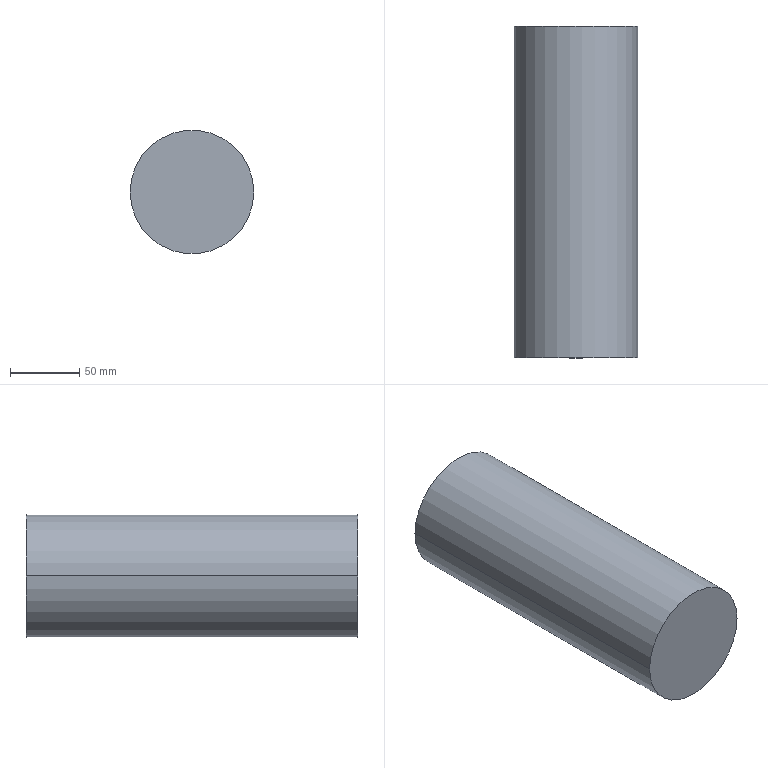Part | STEP file | 1 solid | 7 faces | box 89.417 x 240 x 89.417 mm | volume 636634 mm3 | cylinder 4 | plane 3 | commonest cylinder face diameters 69.417 x2 89.417 x2
STEP:
#1=CARTESIAN_POINT('',(0.,0.,0.));
#2=DIRECTION('',(0.,0.,1.));
#3=DIRECTION('',(1.,0.,0.));
#4=AXIS2_PLACEMENT_3D('',#1,#2,#3);
#5=CARTESIAN_POINT('',(677.16,51.164,248.078));
#6=VERTEX_POINT('',#5);
#7=CARTESIAN_POINT('',(677.16,-178.836,248.078));
#8=VERTEX_POINT('',#7);
#9=CARTESIAN_POINT('',(677.16,51.164,248.078));
#10=DIRECTION('',(0.,-1.,0.));
#11=VECTOR('',#10,1.);
#12=LINE('',#9,#11);
#13=CARTESIAN_POINT('',(642.452,51.164,248.078));
#14=DIRECTION('',(0.,-1.,0.));
#15=DIRECTION('',(1.,0.,0.));
#16=AXIS2_PLACEMENT_3D('',#13,#14,#15);
#17=CYLINDRICAL_SURFACE('',#16,34.708);
#18=CARTESIAN_POINT('',(6.283,0.));
#19=DIRECTION('',(0.,1.));
#20=VECTOR('',#19,1.);
#21=LINE('',#18,#20);
#22=(GEOMETRIC_REPRESENTATION_CONTEXT(2)PARAMETRIC_REPRESENTATION_CONTEXT()REPRESENTATION_CONTEXT('',''));
#23=DEFINITIONAL_REPRESENTATION('',(#21),#22);
#24=PCURVE('',#17,#23);
#25=CARTESIAN_POINT('',(642.452,51.164,248.078));
#26=DIRECTION('',(0.,-1.,0.));
#27=DIRECTION('',(1.,0.,0.));
#28=AXIS2_PLACEMENT_3D('',#25,#26,#27);
#29=CYLINDRICAL_SURFACE('',#28,34.708);
#30=CARTESIAN_POINT('',(0.,0.));
#31=DIRECTION('',(0.,1.));
#32=VECTOR('',#31,1.);
#33=LINE('',#30,#32);
#34=(GEOMETRIC_REPRESENTATION_CONTEXT(2)PARAMETRIC_REPRESENTATION_CONTEXT()REPRESENTATION_CONTEXT('',''));
#35=DEFINITIONAL_REPRESENTATION('',(#33),#34);
#36=PCURVE('',#29,#35);
#37=SURFACE_CURVE('',#12,(#24,#36),.PCURVE_S1.);
#38=EDGE_CURVE('',#6,#8,#37,.T.);
#39=ORIENTED_EDGE('',*,*,#38,.T.);
#40=CARTESIAN_POINT('',(607.743,-178.836,248.078));
#41=VERTEX_POINT('',#40);
#42=CARTESIAN_POINT('',(642.452,-178.836,248.078));
#43=DIRECTION('',(0.,1.,0.));
#44=DIRECTION('',(-1.,0.,0.));
#45=AXIS2_PLACEMENT_3D('',#42,#43,#44);
#46=CIRCLE('',#45,34.708);
#47=CARTESIAN_POINT('',(9.425,230.));
#48=DIRECTION('',(-1.,0.));
#49=VECTOR('',#48,1.);
#50=LINE('',#47,#49);
#51=(GEOMETRIC_REPRESENTATION_CONTEXT(2)PARAMETRIC_REPRESENTATION_CONTEXT()REPRESENTATION_CONTEXT('',''));
#52=DEFINITIONAL_REPRESENTATION('',(#50),#51);
#53=PCURVE('',#17,#52);
#54=CARTESIAN_POINT('',(642.452,-178.836,248.078));
#55=DIRECTION('',(0.,1.,0.));
#56=DIRECTION('',(-1.,0.,0.));
#57=AXIS2_PLACEMENT_3D('',#54,#55,#56);
#58=PLANE('',#57);
#59=CARTESIAN_POINT('',(0.,0.));
#60=DIRECTION('',(1.,0.));
#61=AXIS2_PLACEMENT_2D('',#59,#60);
#62=CIRCLE('',#61,34.708);
#63=(GEOMETRIC_REPRESENTATION_CONTEXT(2)PARAMETRIC_REPRESENTATION_CONTEXT()REPRESENTATION_CONTEXT('',''));
#64=DEFINITIONAL_REPRESENTATION('',(#62),#63);
#65=PCURVE('',#58,#64);
#66=SURFACE_CURVE('',#46,(#53,#65),.PCURVE_S1.);
#67=EDGE_CURVE('',#8,#41,#66,.T.);
#68=ORIENTED_EDGE('',*,*,#67,.T.);
#69=CARTESIAN_POINT('',(607.743,51.164,248.078));
#70=VERTEX_POINT('',#69);
#71=CARTESIAN_POINT('',(607.743,51.164,248.078));
#72=DIRECTION('',(0.,-1.,0.));
#73=VECTOR('',#72,1.);
#74=LINE('',#71,#73);
#75=CARTESIAN_POINT('',(3.142,0.));
#76=DIRECTION('',(0.,1.));
#77=VECTOR('',#76,1.);
#78=LINE('',#75,#77);
#79=(GEOMETRIC_REPRESENTATION_CONTEXT(2)PARAMETRIC_REPRESENTATION_CONTEXT()REPRESENTATION_CONTEXT('',''));
#80=DEFINITIONAL_REPRESENTATION('',(#78),#79);
#81=PCURVE('',#17,#80);
#82=CARTESIAN_POINT('',(3.142,0.));
#83=DIRECTION('',(0.,1.));
#84=VECTOR('',#83,1.);
#85=LINE('',#82,#84);
#86=(GEOMETRIC_REPRESENTATION_CONTEXT(2)PARAMETRIC_REPRESENTATION_CONTEXT()REPRESENTATION_CONTEXT('',''));
#87=DEFINITIONAL_REPRESENTATION('',(#85),#86);
#88=PCURVE('',#29,#87);
#89=SURFACE_CURVE('',#74,(#81,#88),.PCURVE_S1.);
#90=EDGE_CURVE('',#70,#41,#89,.T.);
#91=ORIENTED_EDGE('',*,*,#90,.F.);
#92=CARTESIAN_POINT('',(642.452,51.164,248.078));
#93=DIRECTION('',(0.,1.,0.));
#94=DIRECTION('',(-1.,0.,0.));
#95=AXIS2_PLACEMENT_3D('',#92,#93,#94);
#96=CIRCLE('',#95,34.708);
#97=CARTESIAN_POINT('',(9.425,0.));
#98=DIRECTION('',(-1.,0.));
#99=VECTOR('',#98,1.);
#100=LINE('',#97,#99);
#101=(GEOMETRIC_REPRESENTATION_CONTEXT(2)PARAMETRIC_REPRESENTATION_CONTEXT()REPRESENTATION_CONTEXT('',''));
#102=DEFINITIONAL_REPRESENTATION('',(#100),#101);
#103=PCURVE('',#17,#102);
#104=CARTESIAN_POINT('',(642.452,51.164,248.078));
#105=DIRECTION('',(0.,1.,0.));
#106=DIRECTION('',(-1.,0.,0.));
#107=AXIS2_PLACEMENT_3D('',#104,#105,#106);
#108=PLANE('',#107);
#109=CARTESIAN_POINT('',(0.,0.));
#110=DIRECTION('',(1.,0.));
#111=AXIS2_PLACEMENT_2D('',#109,#110);
#112=CIRCLE('',#111,34.708);
#113=(GEOMETRIC_REPRESENTATION_CONTEXT(2)PARAMETRIC_REPRESENTATION_CONTEXT()REPRESENTATION_CONTEXT('',''));
#114=DEFINITIONAL_REPRESENTATION('',(#112),#113);
#115=PCURVE('',#108,#114);
#116=SURFACE_CURVE('',#96,(#103,#115),.PCURVE_S1.);
#117=EDGE_CURVE('',#6,#70,#116,.T.);
#118=ORIENTED_EDGE('',*,*,#117,.F.);
#119=EDGE_LOOP('',(#39,#68,#91,#118));
#120=FACE_BOUND('',#119,.F.);
#121=ADVANCED_FACE('',(#120),#17,.F.);
#122=CARTESIAN_POINT('',(597.743,51.164,248.078));
#123=VERTEX_POINT('',#122);
#124=CARTESIAN_POINT('',(687.16,51.164,248.078));
#125=VERTEX_POINT('',#124);
#126=CARTESIAN_POINT('',(642.452,51.164,248.078));
#127=DIRECTION('',(0.,1.,0.));
#128=DIRECTION('',(-1.,0.,0.));
#129=AXIS2_PLACEMENT_3D('',#126,#127,#128);
#130=CIRCLE('',#129,44.708);
#131=CARTESIAN_POINT('',(642.452,51.164,248.078));
#132=DIRECTION('',(0.,-1.,0.));
#133=DIRECTION('',(1.,0.,0.));
#134=AXIS2_PLACEMENT_3D('',#131,#132,#133);
#135=CYLINDRICAL_SURFACE('',#134,44.708);
#136=CARTESIAN_POINT('',(3.142,0.));
#137=DIRECTION('',(-1.,0.));
#138=VECTOR('',#137,1.);
#139=LINE('',#136,#138);
#140=(GEOMETRIC_REPRESENTATION_CONTEXT(2)PARAMETRIC_REPRESENTATION_CONTEXT()REPRESENTATION_CONTEXT('',''));
#141=DEFINITIONAL_REPRESENTATION('',(#139),#140);
#142=PCURVE('',#135,#141);
#143=CARTESIAN_POINT('',(0.,0.));
#144=DIRECTION('',(1.,0.));
#145=AXIS2_PLACEMENT_2D('',#143,#144);
#146=CIRCLE('',#145,44.708);
#147=(GEOMETRIC_REPRESENTATION_CONTEXT(2)PARAMETRIC_REPRESENTATION_CONTEXT()REPRESENTATION_CONTEXT('',''));
#148=DEFINITIONAL_REPRESENTATION('',(#146),#147);
#149=PCURVE('',#108,#148);
#150=SURFACE_CURVE('',#130,(#142,#149),.PCURVE_S1.);
#151=EDGE_CURVE('',#123,#125,#150,.T.);
#152=ORIENTED_EDGE('',*,*,#151,.F.);
#153=CARTESIAN_POINT('',(597.743,-188.836,248.078));
#154=VERTEX_POINT('',#153);
#155=CARTESIAN_POINT('',(597.743,51.164,248.078));
#156=DIRECTION('',(0.,-1.,0.));
#157=VECTOR('',#156,1.);
#158=LINE('',#155,#157);
#159=CARTESIAN_POINT('',(3.142,0.));
#160=DIRECTION('',(0.,1.));
#161=VECTOR('',#160,1.);
#162=LINE('',#159,#161);
#163=(GEOMETRIC_REPRESENTATION_CONTEXT(2)PARAMETRIC_REPRESENTATION_CONTEXT()REPRESENTATION_CONTEXT('',''));
#164=DEFINITIONAL_REPRESENTATION('',(#162),#163);
#165=PCURVE('',#135,#164);
#166=CARTESIAN_POINT('',(642.452,51.164,248.078));
#167=DIRECTION('',(0.,-1.,0.));
#168=DIRECTION('',(1.,0.,0.));
#169=AXIS2_PLACEMENT_3D('',#166,#167,#168);
#170=CYLINDRICAL_SURFACE('',#169,44.708);
#171=CARTESIAN_POINT('',(3.142,0.));
#172=DIRECTION('',(0.,1.));
#173=VECTOR('',#172,1.);
#174=LINE('',#171,#173);
#175=(GEOMETRIC_REPRESENTATION_CONTEXT(2)PARAMETRIC_REPRESENTATION_CONTEXT()REPRESENTATION_CONTEXT('',''));
#176=DEFINITIONAL_REPRESENTATION('',(#174),#175);
#177=PCURVE('',#170,#176);
#178=SURFACE_CURVE('',#158,(#165,#177),.PCURVE_S1.);
#179=EDGE_CURVE('',#123,#154,#178,.T.);
#180=ORIENTED_EDGE('',*,*,#179,.T.);
#181=CARTESIAN_POINT('',(687.16,-188.836,248.078));
#182=VERTEX_POINT('',#181);
#183=CARTESIAN_POINT('',(642.452,-188.836,248.078));
#184=DIRECTION('',(0.,1.,0.));
#185=DIRECTION('',(-1.,0.,0.));
#186=AXIS2_PLACEMENT_3D('',#183,#184,#185);
#187=CIRCLE('',#186,44.708);
#188=CARTESIAN_POINT('',(3.142,240.));
#189=DIRECTION('',(-1.,0.));
#190=VECTOR('',#189,1.);
#191=LINE('',#188,#190);
#192=(GEOMETRIC_REPRESENTATION_CONTEXT(2)PARAMETRIC_REPRESENTATION_CONTEXT()REPRESENTATION_CONTEXT('',''));
#193=DEFINITIONAL_REPRESENTATION('',(#191),#192);
#194=PCURVE('',#135,#193);
#195=CARTESIAN_POINT('',(642.452,-188.836,248.078));
#196=DIRECTION('',(0.,1.,0.));
#197=DIRECTION('',(-1.,0.,0.));
#198=AXIS2_PLACEMENT_3D('',#195,#196,#197);
#199=PLANE('',#198);
#200=CARTESIAN_POINT('',(0.,0.));
#201=DIRECTION('',(1.,0.));
#202=AXIS2_PLACEMENT_2D('',#200,#201);
#203=CIRCLE('',#202,44.708);
#204=(GEOMETRIC_REPRESENTATION_CONTEXT(2)PARAMETRIC_REPRESENTATION_CONTEXT()REPRESENTATION_CONTEXT('',''));
#205=DEFINITIONAL_REPRESENTATION('',(#203),#204);
#206=PCURVE('',#199,#205);
#207=SURFACE_CURVE('',#187,(#194,#206),.PCURVE_S1.);
#208=EDGE_CURVE('',#154,#182,#207,.T.);
#209=ORIENTED_EDGE('',*,*,#208,.T.);
#210=CARTESIAN_POINT('',(687.16,51.164,248.078));
#211=DIRECTION('',(0.,-1.,0.));
#212=VECTOR('',#211,1.);
#213=LINE('',#210,#212);
#214=CARTESIAN_POINT('',(0.,0.));
#215=DIRECTION('',(0.,1.));
#216=VECTOR('',#215,1.);
#217=LINE('',#214,#216);
#218=(GEOMETRIC_REPRESENTATION_CONTEXT(2)PARAMETRIC_REPRESENTATION_CONTEXT()REPRESENTATION_CONTEXT('',''));
#219=DEFINITIONAL_REPRESENTATION('',(#217),#218);
#220=PCURVE('',#135,#219);
#221=CARTESIAN_POINT('',(6.283,0.));
#222=DIRECTION('',(0.,1.));
#223=VECTOR('',#222,1.);
#224=LINE('',#221,#223);
#225=(GEOMETRIC_REPRESENTATION_CONTEXT(2)PARAMETRIC_REPRESENTATION_CONTEXT()REPRESENTATION_CONTEXT('',''));
#226=DEFINITIONAL_REPRESENTATION('',(#224),#225);
#227=PCURVE('',#170,#226);
#228=SURFACE_CURVE('',#213,(#220,#227),.PCURVE_S1.);
#229=EDGE_CURVE('',#125,#182,#228,.T.);
#230=ORIENTED_EDGE('',*,*,#229,.F.);
#231=EDGE_LOOP('',(#152,#180,#209,#230));
#232=FACE_BOUND('',#231,.T.);
#233=ADVANCED_FACE('',(#232),#135,.T.);
#234=ORIENTED_EDGE('',*,*,#179,.F.);
#235=CARTESIAN_POINT('',(642.452,51.164,248.078));
#236=DIRECTION('',(0.,1.,0.));
#237=DIRECTION('',(-1.,0.,0.));
#238=AXIS2_PLACEMENT_3D('',#235,#236,#237);
#239=CIRCLE('',#238,44.708);
#240=CARTESIAN_POINT('',(9.425,0.));
#241=DIRECTION('',(-1.,0.));
#242=VECTOR('',#241,1.);
#243=LINE('',#240,#242);
#244=(GEOMETRIC_REPRESENTATION_CONTEXT(2)PARAMETRIC_REPRESENTATION_CONTEXT()REPRESENTATION_CONTEXT('',''));
#245=DEFINITIONAL_REPRESENTATION('',(#243),#244);
#246=PCURVE('',#170,#245);
#247=CARTESIAN_POINT('',(0.,0.));
#248=DIRECTION('',(1.,0.));
#249=AXIS2_PLACEMENT_2D('',#247,#248);
#250=CIRCLE('',#249,44.708);
#251=(GEOMETRIC_REPRESENTATION_CONTEXT(2)PARAMETRIC_REPRESENTATION_CONTEXT()REPRESENTATION_CONTEXT('',''));
#252=DEFINITIONAL_REPRESENTATION('',(#250),#251);
#253=PCURVE('',#108,#252);
#254=SURFACE_CURVE('',#239,(#246,#253),.PCURVE_S1.);
#255=EDGE_CURVE('',#125,#123,#254,.T.);
#256=ORIENTED_EDGE('',*,*,#255,.F.);
#257=ORIENTED_EDGE('',*,*,#229,.T.);
#258=CARTESIAN_POINT('',(642.452,-188.836,248.078));
#259=DIRECTION('',(0.,1.,0.));
#260=DIRECTION('',(-1.,0.,0.));
#261=AXIS2_PLACEMENT_3D('',#258,#259,#260);
#262=CIRCLE('',#261,44.708);
#263=CARTESIAN_POINT('',(9.425,240.));
#264=DIRECTION('',(-1.,0.));
#265=VECTOR('',#264,1.);
#266=LINE('',#263,#265);
#267=(GEOMETRIC_REPRESENTATION_CONTEXT(2)PARAMETRIC_REPRESENTATION_CONTEXT()REPRESENTATION_CONTEXT('',''));
#268=DEFINITIONAL_REPRESENTATION('',(#266),#267);
#269=PCURVE('',#170,#268);
#270=CARTESIAN_POINT('',(0.,0.));
#271=DIRECTION('',(1.,0.));
#272=AXIS2_PLACEMENT_2D('',#270,#271);
#273=CIRCLE('',#272,44.708);
#274=(GEOMETRIC_REPRESENTATION_CONTEXT(2)PARAMETRIC_REPRESENTATION_CONTEXT()REPRESENTATION_CONTEXT('',''));
#275=DEFINITIONAL_REPRESENTATION('',(#273),#274);
#276=PCURVE('',#199,#275);
#277=SURFACE_CURVE('',#262,(#269,#276),.PCURVE_S1.);
#278=EDGE_CURVE('',#182,#154,#277,.T.);
#279=ORIENTED_EDGE('',*,*,#278,.T.);
#280=EDGE_LOOP('',(#234,#256,#257,#279));
#281=FACE_BOUND('',#280,.T.);
#282=ADVANCED_FACE('',(#281),#170,.T.);
#283=ORIENTED_EDGE('',*,*,#117,.F.);
#284=CARTESIAN_POINT('',(642.452,51.164,248.078));
#285=DIRECTION('',(0.,1.,0.));
#286=DIRECTION('',(-1.,0.,0.));
#287=AXIS2_PLACEMENT_3D('',#284,#285,#286);
#288=CIRCLE('',#287,34.708);
#289=CARTESIAN_POINT('',(0.,0.));
#290=DIRECTION('',(1.,0.));
#291=AXIS2_PLACEMENT_2D('',#289,#290);
#292=CIRCLE('',#291,34.708);
#293=(GEOMETRIC_REPRESENTATION_CONTEXT(2)PARAMETRIC_REPRESENTATION_CONTEXT()REPRESENTATION_CONTEXT('',''));
#294=DEFINITIONAL_REPRESENTATION('',(#292),#293);
#295=PCURVE('',#108,#294);
#296=CARTESIAN_POINT('',(3.142,0.));
#297=DIRECTION('',(-1.,0.));
#298=VECTOR('',#297,1.);
#299=LINE('',#296,#298);
#300=(GEOMETRIC_REPRESENTATION_CONTEXT(2)PARAMETRIC_REPRESENTATION_CONTEXT()REPRESENTATION_CONTEXT('',''));
#301=DEFINITIONAL_REPRESENTATION('',(#299),#300);
#302=PCURVE('',#29,#301);
#303=SURFACE_CURVE('',#288,(#295,#302),.PCURVE_S1.);
#304=EDGE_CURVE('',#70,#6,#303,.T.);
#305=ORIENTED_EDGE('',*,*,#304,.F.);
#306=EDGE_LOOP('',(#283,#305));
#307=FACE_BOUND('',#306,.T.);
#308=ORIENTED_EDGE('',*,*,#255,.T.);
#309=ORIENTED_EDGE('',*,*,#151,.T.);
#310=EDGE_LOOP('',(#308,#309));
#311=FACE_BOUND('',#310,.T.);
#312=ADVANCED_FACE('',(#307,#311),#108,.T.);
#313=ORIENTED_EDGE('',*,*,#278,.F.);
#314=ORIENTED_EDGE('',*,*,#208,.F.);
#315=EDGE_LOOP('',(#313,#314));
#316=FACE_BOUND('',#315,.T.);
#317=ADVANCED_FACE('',(#316),#199,.F.);
#318=CARTESIAN_POINT('',(642.452,-178.836,248.078));
#319=DIRECTION('',(0.,1.,0.));
#320=DIRECTION('',(-1.,0.,0.));
#321=AXIS2_PLACEMENT_3D('',#318,#319,#320);
#322=CIRCLE('',#321,34.708);
#323=CARTESIAN_POINT('',(3.142,230.));
#324=DIRECTION('',(-1.,0.));
#325=VECTOR('',#324,1.);
#326=LINE('',#323,#325);
#327=(GEOMETRIC_REPRESENTATION_CONTEXT(2)PARAMETRIC_REPRESENTATION_CONTEXT()REPRESENTATION_CONTEXT('',''));
#328=DEFINITIONAL_REPRESENTATION('',(#326),#327);
#329=PCURVE('',#29,#328);
#330=CARTESIAN_POINT('',(0.,0.));
#331=DIRECTION('',(1.,0.));
#332=AXIS2_PLACEMENT_2D('',#330,#331);
#333=CIRCLE('',#332,34.708);
#334=(GEOMETRIC_REPRESENTATION_CONTEXT(2)PARAMETRIC_REPRESENTATION_CONTEXT()REPRESENTATION_CONTEXT('',''));
#335=DEFINITIONAL_REPRESENTATION('',(#333),#334);
#336=PCURVE('',#58,#335);
#337=SURFACE_CURVE('',#322,(#329,#336),.PCURVE_S1.);
#338=EDGE_CURVE('',#41,#8,#337,.T.);
#339=ORIENTED_EDGE('',*,*,#338,.T.);
#340=ORIENTED_EDGE('',*,*,#38,.F.);
#341=ORIENTED_EDGE('',*,*,#304,.F.);
#342=ORIENTED_EDGE('',*,*,#90,.T.);
#343=EDGE_LOOP('',(#339,#340,#341,#342));
#344=FACE_BOUND('',#343,.F.);
#345=ADVANCED_FACE('',(#344),#29,.F.);
#346=ORIENTED_EDGE('',*,*,#67,.T.);
#347=ORIENTED_EDGE('',*,*,#338,.T.);
#348=EDGE_LOOP('',(#346,#347));
#349=FACE_BOUND('',#348,.T.);
#350=ADVANCED_FACE('',(#349),#58,.T.);
#351=CLOSED_SHELL('',(#121,#233,#282,#312,#317,#345,#350));
#352=MANIFOLD_SOLID_BREP('',#351);
#353=(LENGTH_UNIT()NAMED_UNIT(*)SI_UNIT(.MILLI.,.METRE.));
#354=UNCERTAINTY_MEASURE_WITH_UNIT(LENGTH_MEASURE(0.0000001),#353,'','');
#355=(NAMED_UNIT(*)PLANE_ANGLE_UNIT()SI_UNIT($,.RADIAN.));
#356=(NAMED_UNIT(*)SI_UNIT($,.STERADIAN.)SOLID_ANGLE_UNIT());
#357=(GEOMETRIC_REPRESENTATION_CONTEXT(3)GLOBAL_UNCERTAINTY_ASSIGNED_CONTEXT((#354))GLOBAL_UNIT_ASSIGNED_CONTEXT((#353,#355,#356))REPRESENTATION_CONTEXT('',''));
#358=ADVANCED_BREP_SHAPE_REPRESENTATION('',(#4,#352),#357);